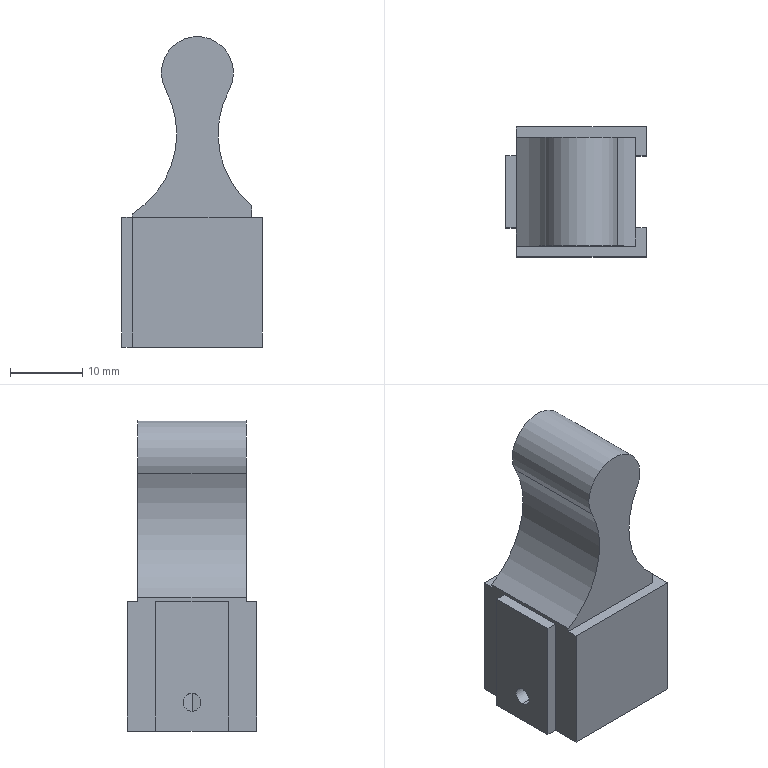Part | STEP file | Seal sleeve 2 | 1 solid | 25 faces | box 19.5 x 18 x 43 mm | volume 8218 mm3 | plane 18 | cylinder 7 | commonest cylinder face diameters 10 x3 2.5 x2 26 x2